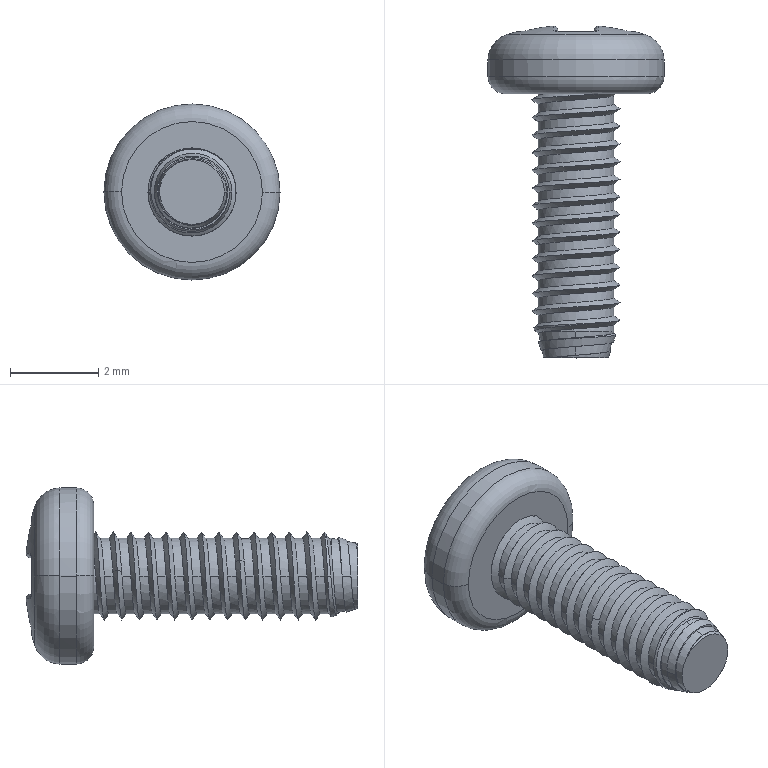Part | SolidWorks | features BaseBody 1 | 1 solid | 115 faces | box 4 x 7.54 x 4 mm | volume 28.459 mm3 | spline 38 | cylinder 35 | cone 15 | plane 11 | torus 8 | sphere 8 | commonest cylinder face diameters 1.713 x29 0.2 x4 4 x2